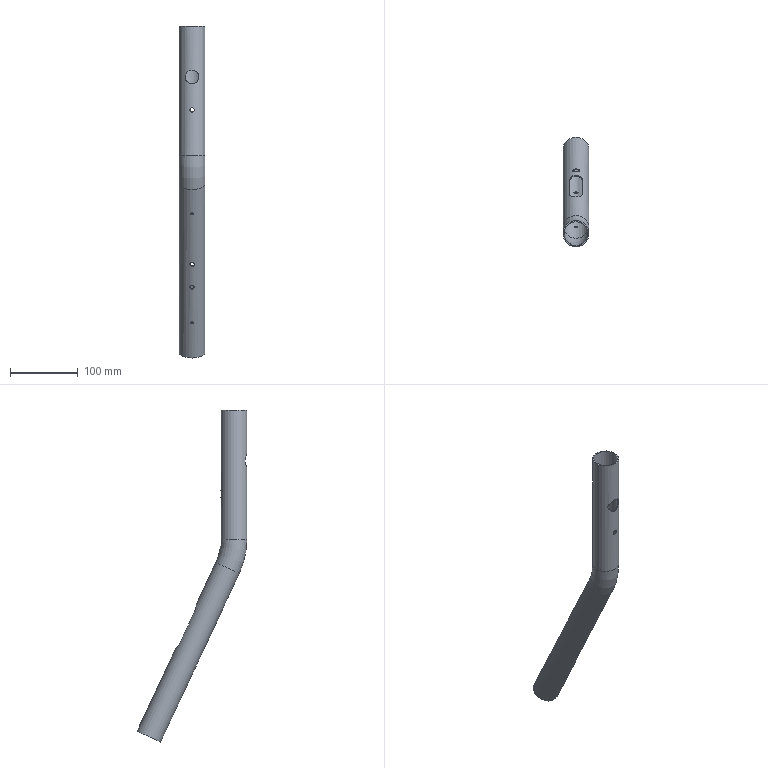Part | STEP file | Q7C1205R | 1 solid | 20 faces | box 38.1 x 161.362 x 488.383 mm | volume 84651 mm3 | cylinder 14 | plane 4 | torus 2 | commonest cylinder face diameters 6.5 x3 3.5 x2 10 x2 18 x2 35.1 x2 38.1 x2